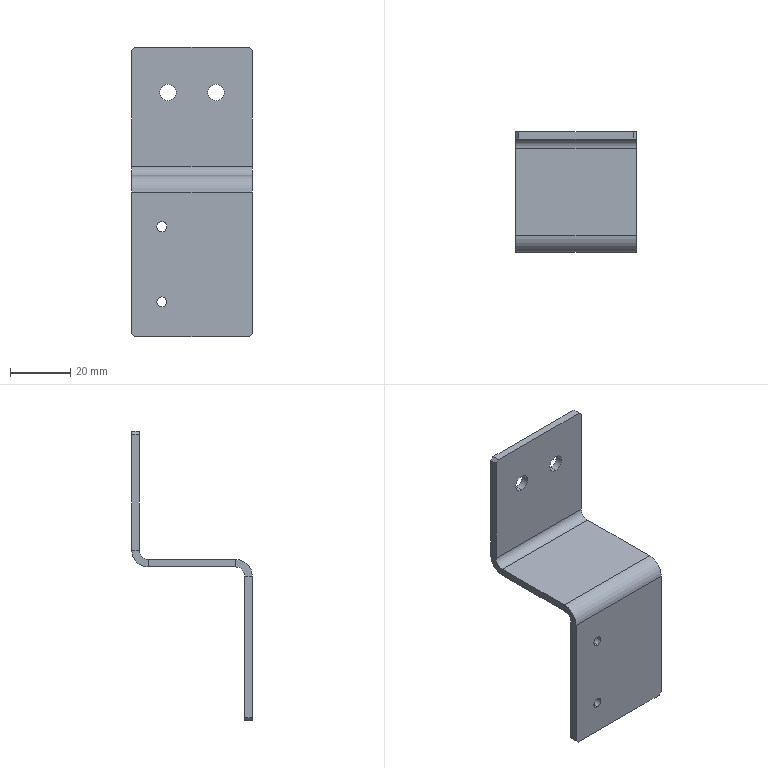Part | STEP file | 227H056255 BKT_Default | 1 solid | 34 faces | box 40 x 40 x 96 mm | volume 12819 mm3 | plane 22 | cylinder 12 | commonest cylinder face diameters 3.3 x4 5.5 x4 6 x2 11 x2